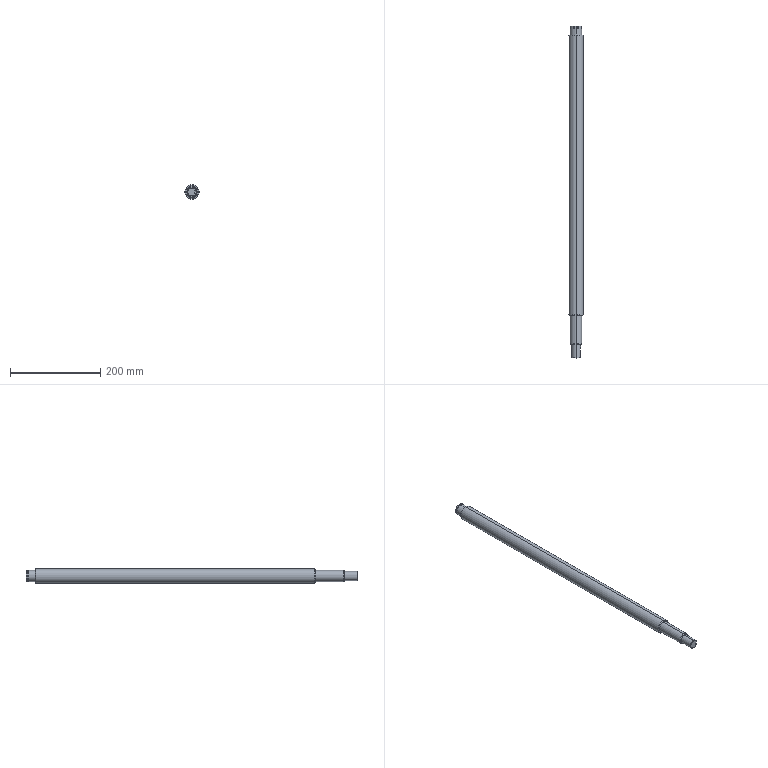Part | SolidWorks | features ICE 4, Chamfer 1, RevCut 1, Revolution 1 | 1 solid | 34 faces | box 32 x 734 x 32 mm | volume 548270 mm3 | cylinder 13 | cone 11 | plane 10 | commonest cylinder face diameters 25 x6 20 x2 23.9 x2 32 x2 6 x1
STEP:
#1=CARTESIAN_POINT('',(0.,344.5,11.5));
#2=VERTEX_POINT('',#1);
#3=CARTESIAN_POINT('',(0.,344.5,-11.5));
#4=VERTEX_POINT('',#3);
#5=CARTESIAN_POINT('',(0.,344.5,0.));
#6=DIRECTION('',(0.,1.,0.));
#7=DIRECTION('',(0.,0.,1.));
#8=AXIS2_PLACEMENT_3D('',#5,#6,#7);
#9=CIRCLE('',#8,11.5);
#10=EDGE_CURVE('',#2,#4,#9,.T.);
#11=ORIENTED_EDGE('',*,*,#10,.F.);
#12=CARTESIAN_POINT('',(0.,343.5,12.5));
#13=VERTEX_POINT('',#12);
#14=CARTESIAN_POINT('',(0.,344.5,11.5));
#15=DIRECTION('',(0.,-0.7071,0.7071));
#16=VECTOR('',#15,1000.);
#17=LINE('',#14,#16);
#18=EDGE_CURVE('',#2,#13,#17,.T.);
#19=ORIENTED_EDGE('',*,*,#18,.T.);
#20=CARTESIAN_POINT('',(0.,343.5,-12.5));
#21=VERTEX_POINT('',#20);
#22=CARTESIAN_POINT('',(0.,343.5,0.));
#23=DIRECTION('',(0.,-1.,0.));
#24=DIRECTION('',(0.,0.,1.));
#25=AXIS2_PLACEMENT_3D('',#22,#23,#24);
#26=CIRCLE('',#25,12.5);
#27=EDGE_CURVE('',#21,#13,#26,.T.);
#28=ORIENTED_EDGE('',*,*,#27,.F.);
#29=CARTESIAN_POINT('',(0.,344.5,-11.5));
#30=DIRECTION('',(0.,-0.7071,-0.7071));
#31=VECTOR('',#30,1000.);
#32=LINE('',#29,#31);
#33=EDGE_CURVE('',#4,#21,#32,.T.);
#34=ORIENTED_EDGE('',*,*,#33,.F.);
#35=EDGE_LOOP('',(#11,#19,#28,#34));
#36=FACE_OUTER_BOUND('',#35,.T.);
#37=CARTESIAN_POINT('',(0.,344.5,0.));
#38=DIRECTION('',(0.,-1.,0.));
#39=DIRECTION('',(0.,0.,-1.));
#40=AXIS2_PLACEMENT_3D('',#37,#38,#39);
#41=CONICAL_SURFACE('',#40,11.5,0.7854);
#42=ADVANCED_FACE('',(#36),#41,.T.);
#43=CARTESIAN_POINT('',(0.,324.5,15.));
#44=VERTEX_POINT('',#43);
#45=CARTESIAN_POINT('',(0.,324.5,-15.));
#46=VERTEX_POINT('',#45);
#47=CARTESIAN_POINT('',(0.,324.5,0.));
#48=DIRECTION('',(0.,1.,0.));
#49=DIRECTION('',(0.,0.,1.));
#50=AXIS2_PLACEMENT_3D('',#47,#48,#49);
#51=CIRCLE('',#50,15.);
#52=EDGE_CURVE('',#44,#46,#51,.T.);
#53=ORIENTED_EDGE('',*,*,#52,.F.);
#54=CARTESIAN_POINT('',(0.,323.5,16.));
#55=VERTEX_POINT('',#54);
#56=CARTESIAN_POINT('',(0.,324.5,15.));
#57=DIRECTION('',(0.,-0.7071,0.7071));
#58=VECTOR('',#57,1000.);
#59=LINE('',#56,#58);
#60=EDGE_CURVE('',#44,#55,#59,.T.);
#61=ORIENTED_EDGE('',*,*,#60,.T.);
#62=CARTESIAN_POINT('',(0.,323.5,-16.));
#63=VERTEX_POINT('',#62);
#64=CARTESIAN_POINT('',(0.,323.5,0.));
#65=DIRECTION('',(0.,-1.,0.));
#66=DIRECTION('',(0.,0.,1.));
#67=AXIS2_PLACEMENT_3D('',#64,#65,#66);
#68=CIRCLE('',#67,16.);
#69=EDGE_CURVE('',#63,#55,#68,.T.);
#70=ORIENTED_EDGE('',*,*,#69,.F.);
#71=CARTESIAN_POINT('',(0.,324.5,-15.));
#72=DIRECTION('',(0.,-0.7071,-0.7071));
#73=VECTOR('',#72,1000.);
#74=LINE('',#71,#73);
#75=EDGE_CURVE('',#46,#63,#74,.T.);
#76=ORIENTED_EDGE('',*,*,#75,.F.);
#77=EDGE_LOOP('',(#53,#61,#70,#76));
#78=FACE_OUTER_BOUND('',#77,.T.);
#79=CARTESIAN_POINT('',(0.,324.5,0.));
#80=DIRECTION('',(0.,-1.,0.));
#81=DIRECTION('',(0.,0.,-1.));
#82=AXIS2_PLACEMENT_3D('',#79,#80,#81);
#83=CONICAL_SURFACE('',#82,15.,0.7854);
#84=ADVANCED_FACE('',(#78),#83,.T.);
#85=CARTESIAN_POINT('',(0.,-294.5,-15.));
#86=VERTEX_POINT('',#85);
#87=CARTESIAN_POINT('',(0.,-294.5,15.));
#88=VERTEX_POINT('',#87);
#89=CARTESIAN_POINT('',(0.,-294.5,0.));
#90=DIRECTION('',(0.,-1.,0.));
#91=DIRECTION('',(0.,0.,-1.));
#92=AXIS2_PLACEMENT_3D('',#89,#90,#91);
#93=CIRCLE('',#92,15.);
#94=EDGE_CURVE('',#86,#88,#93,.T.);
#95=ORIENTED_EDGE('',*,*,#94,.F.);
#96=CARTESIAN_POINT('',(0.,-293.5,-16.));
#97=VERTEX_POINT('',#96);
#98=CARTESIAN_POINT('',(0.,-293.5,-16.));
#99=DIRECTION('',(0.,0.7071,-0.7071));
#100=VECTOR('',#99,1000.);
#101=LINE('',#98,#100);
#102=EDGE_CURVE('',#86,#97,#101,.T.);
#103=ORIENTED_EDGE('',*,*,#102,.T.);
#104=CARTESIAN_POINT('',(0.,-293.5,16.));
#105=VERTEX_POINT('',#104);
#106=CARTESIAN_POINT('',(0.,-293.5,0.));
#107=DIRECTION('',(0.,1.,0.));
#108=DIRECTION('',(0.,0.,-1.));
#109=AXIS2_PLACEMENT_3D('',#106,#107,#108);
#110=CIRCLE('',#109,16.);
#111=EDGE_CURVE('',#105,#97,#110,.T.);
#112=ORIENTED_EDGE('',*,*,#111,.F.);
#113=CARTESIAN_POINT('',(0.,-293.5,16.));
#114=DIRECTION('',(0.,0.7071,0.7071));
#115=VECTOR('',#114,1000.);
#116=LINE('',#113,#115);
#117=EDGE_CURVE('',#88,#105,#116,.T.);
#118=ORIENTED_EDGE('',*,*,#117,.F.);
#119=EDGE_LOOP('',(#95,#103,#112,#118));
#120=FACE_OUTER_BOUND('',#119,.T.);
#121=CARTESIAN_POINT('',(0.,-293.5,0.));
#122=DIRECTION('',(0.,1.,0.));
#123=DIRECTION('',(0.,0.,1.));
#124=AXIS2_PLACEMENT_3D('',#121,#122,#123);
#125=CONICAL_SURFACE('',#124,16.,0.7854);
#126=ADVANCED_FACE('',(#120),#125,.T.);
#127=CARTESIAN_POINT('',(0.,-359.5,-11.5));
#128=VERTEX_POINT('',#127);
#129=CARTESIAN_POINT('',(0.,-359.5,11.5));
#130=VERTEX_POINT('',#129);
#131=CARTESIAN_POINT('',(0.,-359.5,0.));
#132=DIRECTION('',(0.,-1.,0.));
#133=DIRECTION('',(0.,0.,-1.));
#134=AXIS2_PLACEMENT_3D('',#131,#132,#133);
#135=CIRCLE('',#134,11.5);
#136=EDGE_CURVE('',#128,#130,#135,.T.);
#137=ORIENTED_EDGE('',*,*,#136,.F.);
#138=CARTESIAN_POINT('',(0.,-358.5,-12.5));
#139=VERTEX_POINT('',#138);
#140=CARTESIAN_POINT('',(0.,-359.5,-11.5));
#141=DIRECTION('',(0.,0.7071,-0.7071));
#142=VECTOR('',#141,1000.);
#143=LINE('',#140,#142);
#144=EDGE_CURVE('',#128,#139,#143,.T.);
#145=ORIENTED_EDGE('',*,*,#144,.T.);
#146=CARTESIAN_POINT('',(0.,-358.5,12.5));
#147=VERTEX_POINT('',#146);
#148=CARTESIAN_POINT('',(0.,-358.5,0.));
#149=DIRECTION('',(0.,1.,0.));
#150=DIRECTION('',(0.,0.,-1.));
#151=AXIS2_PLACEMENT_3D('',#148,#149,#150);
#152=CIRCLE('',#151,12.5);
#153=EDGE_CURVE('',#147,#139,#152,.T.);
#154=ORIENTED_EDGE('',*,*,#153,.F.);
#155=CARTESIAN_POINT('',(0.,-359.5,11.5));
#156=DIRECTION('',(0.,0.7071,0.7071));
#157=VECTOR('',#156,1000.);
#158=LINE('',#155,#157);
#159=EDGE_CURVE('',#130,#147,#158,.T.);
#160=ORIENTED_EDGE('',*,*,#159,.F.);
#161=EDGE_LOOP('',(#137,#145,#154,#160));
#162=FACE_OUTER_BOUND('',#161,.T.);
#163=CARTESIAN_POINT('',(0.,-359.5,0.));
#164=DIRECTION('',(0.,1.,0.));
#165=DIRECTION('',(0.,0.,1.));
#166=AXIS2_PLACEMENT_3D('',#163,#164,#165);
#167=CONICAL_SURFACE('',#166,11.5,0.7854);
#168=ADVANCED_FACE('',(#162),#167,.T.);
#169=CARTESIAN_POINT('',(0.,-389.5,-9.));
#170=VERTEX_POINT('',#169);
#171=CARTESIAN_POINT('',(8.485,-389.5,-3.));
#172=VERTEX_POINT('',#171);
#173=CARTESIAN_POINT('',(0.,-389.5,0.));
#174=DIRECTION('',(0.,-1.,0.));
#175=DIRECTION('',(0.,0.,-1.));
#176=AXIS2_PLACEMENT_3D('',#173,#174,#175);
#177=CIRCLE('',#176,9.);
#178=EDGE_CURVE('',#170,#172,#177,.T.);
#179=ORIENTED_EDGE('',*,*,#178,.F.);
#180=CARTESIAN_POINT('',(0.,-388.5,-10.));
#181=VERTEX_POINT('',#180);
#182=CARTESIAN_POINT('',(0.,-389.5,-9.));
#183=DIRECTION('',(0.,0.7071,-0.7071));
#184=VECTOR('',#183,1000.);
#185=LINE('',#182,#184);
#186=EDGE_CURVE('',#170,#181,#185,.T.);
#187=ORIENTED_EDGE('',*,*,#186,.T.);
#188=CARTESIAN_POINT('',(9.539,-388.5,-3.));
#189=VERTEX_POINT('',#188);
#190=CARTESIAN_POINT('',(0.,-388.5,0.));
#191=DIRECTION('',(0.,1.,0.));
#192=DIRECTION('',(0.,0.,-1.));
#193=AXIS2_PLACEMENT_3D('',#190,#191,#192);
#194=CIRCLE('',#193,10.);
#195=EDGE_CURVE('',#189,#181,#194,.T.);
#196=ORIENTED_EDGE('',*,*,#195,.F.);
#197=CARTESIAN_POINT('',(8.485,-389.5,-3.));
#198=CARTESIAN_POINT('',(8.838,-389.168,-3.));
#199=CARTESIAN_POINT('',(9.189,-388.834,-3.));
#200=CARTESIAN_POINT('',(9.539,-388.5,-3.));
#201=B_SPLINE_CURVE_WITH_KNOTS('',3,(#197,#198,#199,#200),.UNSPECIFIED.,.F.,.F.,(4,4),(0.006491,0.007944),.UNSPECIFIED.);
#202=EDGE_CURVE('',#172,#189,#201,.T.);
#203=ORIENTED_EDGE('',*,*,#202,.F.);
#204=EDGE_LOOP('',(#179,#187,#196,#203));
#205=FACE_OUTER_BOUND('',#204,.T.);
#206=CARTESIAN_POINT('',(0.,-389.5,0.));
#207=DIRECTION('',(0.,1.,0.));
#208=DIRECTION('',(0.,0.,1.));
#209=AXIS2_PLACEMENT_3D('',#206,#207,#208);
#210=CONICAL_SURFACE('',#209,9.,0.7854);
#211=ADVANCED_FACE('',(#205),#210,.T.);
#212=ORIENTED_EDGE('',*,*,#186,.F.);
#213=CARTESIAN_POINT('',(0.,-389.5,9.));
#214=VERTEX_POINT('',#213);
#215=CARTESIAN_POINT('',(0.,-389.5,0.));
#216=DIRECTION('',(0.,-1.,0.));
#217=DIRECTION('',(0.,0.,-1.));
#218=AXIS2_PLACEMENT_3D('',#215,#216,#217);
#219=CIRCLE('',#218,9.);
#220=EDGE_CURVE('',#214,#170,#219,.T.);
#221=ORIENTED_EDGE('',*,*,#220,.F.);
#222=CARTESIAN_POINT('',(0.,-388.5,10.));
#223=VERTEX_POINT('',#222);
#224=CARTESIAN_POINT('',(0.,-389.5,9.));
#225=DIRECTION('',(0.,0.7071,0.7071));
#226=VECTOR('',#225,1000.);
#227=LINE('',#224,#226);
#228=EDGE_CURVE('',#214,#223,#227,.T.);
#229=ORIENTED_EDGE('',*,*,#228,.T.);
#230=CARTESIAN_POINT('',(0.,-388.5,0.));
#231=DIRECTION('',(0.,1.,0.));
#232=DIRECTION('',(0.,0.,-1.));
#233=AXIS2_PLACEMENT_3D('',#230,#231,#232);
#234=CIRCLE('',#233,10.);
#235=EDGE_CURVE('',#181,#223,#234,.T.);
#236=ORIENTED_EDGE('',*,*,#235,.F.);
#237=EDGE_LOOP('',(#212,#221,#229,#236));
#238=FACE_OUTER_BOUND('',#237,.T.);
#239=CARTESIAN_POINT('',(0.,-389.5,0.));
#240=DIRECTION('',(0.,1.,0.));
#241=DIRECTION('',(0.,0.,1.));
#242=AXIS2_PLACEMENT_3D('',#239,#240,#241);
#243=CONICAL_SURFACE('',#242,9.,0.7854);
#244=ADVANCED_FACE('',(#238),#243,.T.);
#245=ORIENTED_EDGE('',*,*,#27,.T.);
#246=CARTESIAN_POINT('',(0.,340.85,12.5));
#247=VERTEX_POINT('',#246);
#248=CARTESIAN_POINT('',(0.,344.5,12.5));
#249=DIRECTION('',(0.,-1.,0.));
#250=VECTOR('',#249,1000.);
#251=LINE('',#248,#250);
#252=EDGE_CURVE('',#13,#247,#251,.T.);
#253=ORIENTED_EDGE('',*,*,#252,.T.);
#254=CARTESIAN_POINT('',(0.,340.85,-12.5));
#255=VERTEX_POINT('',#254);
#256=CARTESIAN_POINT('',(0.,340.85,0.));
#257=DIRECTION('',(0.,1.,0.));
#258=DIRECTION('',(0.,0.,1.));
#259=AXIS2_PLACEMENT_3D('',#256,#257,#258);
#260=CIRCLE('',#259,12.5);
#261=EDGE_CURVE('',#247,#255,#260,.T.);
#262=ORIENTED_EDGE('',*,*,#261,.T.);
#263=CARTESIAN_POINT('',(0.,344.5,-12.5));
#264=DIRECTION('',(0.,-1.,0.));
#265=VECTOR('',#264,1000.);
#266=LINE('',#263,#265);
#267=EDGE_CURVE('',#21,#255,#266,.T.);
#268=ORIENTED_EDGE('',*,*,#267,.F.);
#269=EDGE_LOOP('',(#245,#253,#262,#268));
#270=FACE_OUTER_BOUND('',#269,.T.);
#271=CARTESIAN_POINT('',(0.,344.5,0.));
#272=DIRECTION('',(0.,-1.,0.));
#273=DIRECTION('',(0.,0.,-1.));
#274=AXIS2_PLACEMENT_3D('',#271,#272,#273);
#275=CYLINDRICAL_SURFACE('',#274,12.5);
#276=ADVANCED_FACE('',(#270),#275,.T.);
#277=CARTESIAN_POINT('',(0.,340.85,-11.95));
#278=VERTEX_POINT('',#277);
#279=CARTESIAN_POINT('',(0.,340.85,11.95));
#280=VERTEX_POINT('',#279);
#281=CARTESIAN_POINT('',(0.,340.85,0.));
#282=DIRECTION('',(0.,-1.,0.));
#283=DIRECTION('',(0.,0.,-1.));
#284=AXIS2_PLACEMENT_3D('',#281,#282,#283);
#285=CIRCLE('',#284,11.95);
#286=EDGE_CURVE('',#278,#280,#285,.T.);
#287=ORIENTED_EDGE('',*,*,#286,.T.);
#288=CARTESIAN_POINT('',(0.,339.5,11.95));
#289=VERTEX_POINT('',#288);
#290=CARTESIAN_POINT('',(0.,0.,11.95));
#291=DIRECTION('',(0.,-1.,0.));
#292=VECTOR('',#291,1000.);
#293=LINE('',#290,#292);
#294=EDGE_CURVE('',#280,#289,#293,.T.);
#295=ORIENTED_EDGE('',*,*,#294,.T.);
#296=CARTESIAN_POINT('',(0.,339.5,-11.95));
#297=VERTEX_POINT('',#296);
#298=CARTESIAN_POINT('',(0.,339.5,0.));
#299=DIRECTION('',(0.,-1.,0.));
#300=DIRECTION('',(0.,0.,-1.));
#301=AXIS2_PLACEMENT_3D('',#298,#299,#300);
#302=CIRCLE('',#301,11.95);
#303=EDGE_CURVE('',#297,#289,#302,.T.);
#304=ORIENTED_EDGE('',*,*,#303,.F.);
#305=CARTESIAN_POINT('',(0.,0.,-11.95));
#306=DIRECTION('',(0.,-1.,0.));
#307=VECTOR('',#306,1000.);
#308=LINE('',#305,#307);
#309=EDGE_CURVE('',#278,#297,#308,.T.);
#310=ORIENTED_EDGE('',*,*,#309,.F.);
#311=EDGE_LOOP('',(#287,#295,#304,#310));
#312=FACE_OUTER_BOUND('',#311,.T.);
#313=CARTESIAN_POINT('',(0.,0.,0.));
#314=DIRECTION('',(0.,-1.,0.));
#315=DIRECTION('',(0.,0.,-1.));
#316=AXIS2_PLACEMENT_3D('',#313,#314,#315);
#317=CYLINDRICAL_SURFACE('',#316,11.95);
#318=ADVANCED_FACE('',(#312),#317,.T.);
#319=ORIENTED_EDGE('',*,*,#195,.T.);
#320=CARTESIAN_POINT('',(0.,-359.5,-10.));
#321=VERTEX_POINT('',#320);
#322=CARTESIAN_POINT('',(0.,-389.5,-10.));
#323=DIRECTION('',(0.,1.,0.));
#324=VECTOR('',#323,1000.);
#325=LINE('',#322,#324);
#326=EDGE_CURVE('',#181,#321,#325,.T.);
#327=ORIENTED_EDGE('',*,*,#326,.T.);
#328=CARTESIAN_POINT('',(0.,-359.5,10.));
#329=VERTEX_POINT('',#328);
#330=CARTESIAN_POINT('',(0.,-359.5,0.));
#331=DIRECTION('',(0.,-1.,0.));
#332=DIRECTION('',(0.,0.,-1.));
#333=AXIS2_PLACEMENT_3D('',#330,#331,#332);
#334=CIRCLE('',#333,10.);
#335=EDGE_CURVE('',#321,#329,#334,.T.);
#336=ORIENTED_EDGE('',*,*,#335,.T.);
#337=CARTESIAN_POINT('',(0.,-389.5,10.));
#338=DIRECTION('',(0.,1.,0.));
#339=VECTOR('',#338,1000.);
#340=LINE('',#337,#339);
#341=EDGE_CURVE('',#223,#329,#340,.T.);
#342=ORIENTED_EDGE('',*,*,#341,.F.);
#343=CARTESIAN_POINT('',(9.539,-388.5,3.));
#344=VERTEX_POINT('',#343);
#345=CARTESIAN_POINT('',(0.,-388.5,0.));
#346=DIRECTION('',(0.,1.,0.));
#347=DIRECTION('',(0.,0.,-1.));
#348=AXIS2_PLACEMENT_3D('',#345,#346,#347);
#349=CIRCLE('',#348,10.);
#350=EDGE_CURVE('',#223,#344,#349,.T.);
#351=ORIENTED_EDGE('',*,*,#350,.T.);
#352=CARTESIAN_POINT('',(9.539,-369.5,3.));
#353=VERTEX_POINT('',#352);
#354=CARTESIAN_POINT('',(9.539,-389.5,3.));
#355=DIRECTION('',(0.,1.,0.));
#356=VECTOR('',#355,1000.);
#357=LINE('',#354,#356);
#358=EDGE_CURVE('',#344,#353,#357,.T.);
#359=ORIENTED_EDGE('',*,*,#358,.T.);
#360=CARTESIAN_POINT('',(9.539,-369.5,-3.));
#361=VERTEX_POINT('',#360);
#362=CARTESIAN_POINT('',(9.539,-369.5,3.));
#363=CARTESIAN_POINT('',(9.539,-369.301,3.));
#364=CARTESIAN_POINT('',(9.546,-369.105,2.98));
#365=CARTESIAN_POINT('',(9.569,-368.72,2.903));
#366=CARTESIAN_POINT('',(9.587,-368.529,2.845));
#367=CARTESIAN_POINT('',(9.631,-368.166,2.694));
#368=CARTESIAN_POINT('',(9.656,-367.994,2.602));
#369=CARTESIAN_POINT('',(9.712,-367.669,2.385));
#370=CARTESIAN_POINT('',(9.743,-367.516,2.259));
#371=CARTESIAN_POINT('',(9.832,-367.104,1.847));
#372=CARTESIAN_POINT('',(9.891,-366.881,1.514));
#373=CARTESIAN_POINT('',(9.954,-366.656,0.9732));
#374=CARTESIAN_POINT('',(9.971,-366.597,0.783));
#375=CARTESIAN_POINT('',(9.994,-366.52,0.3953));
#376=CARTESIAN_POINT('',(10.,-366.5,0.1999));
#377=CARTESIAN_POINT('',(10.,-366.5,-0.194));
#378=CARTESIAN_POINT('',(9.994,-366.519,-0.394));
#379=CARTESIAN_POINT('',(9.971,-366.596,-0.7797));
#380=CARTESIAN_POINT('',(9.955,-366.653,-0.9673));
#381=CARTESIAN_POINT('',(9.913,-366.805,-1.332));
#382=CARTESIAN_POINT('',(9.887,-366.898,-1.506));
#383=CARTESIAN_POINT('',(9.833,-367.114,-1.83));
#384=CARTESIAN_POINT('',(9.803,-367.24,-1.982));
#385=CARTESIAN_POINT('',(9.743,-367.516,-2.259));
#386=CARTESIAN_POINT('',(9.713,-367.667,-2.383));
#387=CARTESIAN_POINT('',(9.657,-367.99,-2.6));
#388=CARTESIAN_POINT('',(9.631,-368.166,-2.694));
#389=CARTESIAN_POINT('',(9.587,-368.527,-2.845));
#390=CARTESIAN_POINT('',(9.57,-368.714,-2.902));
#391=CARTESIAN_POINT('',(9.546,-369.101,-2.98));
#392=CARTESIAN_POINT('',(9.539,-369.301,-3.));
#393=CARTESIAN_POINT('',(9.539,-369.5,-3.));
#394=B_SPLINE_CURVE_WITH_KNOTS('',3,(#362,#363,#364,#365,#366,#367,#368,#369,#370,#371,#372,#373,#374,#375,#376,#377,#378,#379,#380,#381,#382,#383,#384,#385,#386,#387,#388,#389,#390,#391,#392,#393),.UNSPECIFIED.,.F.,.F.,(4,2,2,2,2,2,2,2,2,2,2,2,2,2,2,4),(0.,0.0005894,0.001179,0.001768,0.002358,0.003536,0.004126,0.004715,0.005305,0.005894,0.006484,0.007073,0.007662,0.008252,0.008841,0.009431),.UNSPECIFIED.);
#395=EDGE_CURVE('',#353,#361,#394,.T.);
#396=ORIENTED_EDGE('',*,*,#395,.T.);
#397=CARTESIAN_POINT('',(9.539,-389.5,-3.));
#398=DIRECTION('',(0.,-1.,0.));
#399=VECTOR('',#398,1000.);
#400=LINE('',#397,#399);
#401=EDGE_CURVE('',#361,#189,#400,.T.);
#402=ORIENTED_EDGE('',*,*,#401,.T.);
#403=EDGE_LOOP('',(#319,#327,#336,#342,#351,#359,#396,#402));
#404=FACE_OUTER_BOUND('',#403,.T.);
#405=CARTESIAN_POINT('',(0.,-389.5,0.));
#406=DIRECTION('',(0.,1.,0.));
#407=DIRECTION('',(0.,0.,1.));
#408=AXIS2_PLACEMENT_3D('',#405,#406,#407);
#409=CYLINDRICAL_SURFACE('',#408,10.);
#410=ADVANCED_FACE('',(#404),#409,.T.);
#411=ORIENTED_EDGE('',*,*,#153,.T.);
#412=CARTESIAN_POINT('',(0.,-294.5,-12.5));
#413=VERTEX_POINT('',#412);
#414=CARTESIAN_POINT('',(0.,-359.5,-12.5));
#415=DIRECTION('',(0.,1.,0.));
#416=VECTOR('',#415,1000.);
#417=LINE('',#414,#416);
#418=EDGE_CURVE('',#139,#413,#417,.T.);
#419=ORIENTED_EDGE('',*,*,#418,.T.);
#420=CARTESIAN_POINT('',(0.,-294.5,12.5));
#421=VERTEX_POINT('',#420);
#422=CARTESIAN_POINT('',(0.,-294.5,0.));
#423=DIRECTION('',(0.,-1.,0.));
#424=DIRECTION('',(0.,0.,-1.));
#425=AXIS2_PLACEMENT_3D('',#422,#423,#424);
#426=CIRCLE('',#425,12.5);
#427=EDGE_CURVE('',#413,#421,#426,.T.);
#428=ORIENTED_EDGE('',*,*,#427,.T.);
#429=CARTESIAN_POINT('',(0.,-359.5,12.5));
#430=DIRECTION('',(0.,1.,0.));
#431=VECTOR('',#430,1000.);
#432=LINE('',#429,#431);
#433=EDGE_CURVE('',#147,#421,#432,.T.);
#434=ORIENTED_EDGE('',*,*,#433,.F.);
#435=EDGE_LOOP('',(#411,#419,#428,#434));
#436=FACE_OUTER_BOUND('',#435,.T.);
#437=CARTESIAN_POINT('',(0.,-359.5,0.));
#438=DIRECTION('',(0.,1.,0.));
#439=DIRECTION('',(0.,0.,1.));
#440=AXIS2_PLACEMENT_3D('',#437,#438,#439);
#441=CYLINDRICAL_SURFACE('',#440,12.5);
#442=ADVANCED_FACE('',(#436),#441,.T.);
#443=ORIENTED_EDGE('',*,*,#111,.T.);
#444=CARTESIAN_POINT('',(0.,-294.5,-16.));
#445=DIRECTION('',(0.,1.,0.));
#446=VECTOR('',#445,1000.);
#447=LINE('',#444,#446);
#448=EDGE_CURVE('',#97,#63,#447,.T.);
#449=ORIENTED_EDGE('',*,*,#448,.T.);
#450=ORIENTED_EDGE('',*,*,#69,.T.);
#451=CARTESIAN_POINT('',(0.,-294.5,16.));
#452=DIRECTION('',(0.,1.,0.));
#453=VECTOR('',#452,1000.);
#454=LINE('',#451,#453);
#455=EDGE_CURVE('',#105,#55,#454,.T.);
#456=ORIENTED_EDGE('',*,*,#455,.F.);
#457=EDGE_LOOP('',(#443,#449,#450,#456));
#458=FACE_OUTER_BOUND('',#457,.T.);
#459=CARTESIAN_POINT('',(0.,-294.5,0.));
#460=DIRECTION('',(0.,1.,0.));
#461=DIRECTION('',(0.,0.,1.));
#462=AXIS2_PLACEMENT_3D('',#459,#460,#461);
#463=CYLINDRICAL_SURFACE('',#462,16.);
#464=ADVANCED_FACE('',(#458),#463,.T.);
#465=CARTESIAN_POINT('',(0.,339.5,-12.5));
#466=VERTEX_POINT('',#465);
#467=CARTESIAN_POINT('',(0.,339.5,12.5));
#468=VERTEX_POINT('',#467);
#469=CARTESIAN_POINT('',(0.,339.5,0.));
#470=DIRECTION('',(0.,-1.,0.));
#471=DIRECTION('',(0.,0.,-1.));
#472=AXIS2_PLACEMENT_3D('',#469,#470,#471);
#473=CIRCLE('',#472,12.5);
#474=EDGE_CURVE('',#466,#468,#473,.T.);
#475=ORIENTED_EDGE('',*,*,#474,.T.);
#476=CARTESIAN_POINT('',(0.,324.5,12.5));
#477=VERTEX_POINT('',#476);
#478=CARTESIAN_POINT('',(0.,344.5,12.5));
#479=DIRECTION('',(0.,-1.,0.));
#480=VECTOR('',#479,1000.);
#481=LINE('',#478,#480);
#482=EDGE_CURVE('',#468,#477,#481,.T.);
#483=ORIENTED_EDGE('',*,*,#482,.T.);
#484=CARTESIAN_POINT('',(0.,324.5,-12.5));
#485=VERTEX_POINT('',#484);
#486=CARTESIAN_POINT('',(0.,324.5,0.));
#487=DIRECTION('',(0.,1.,0.));
#488=DIRECTION('',(0.,0.,1.));
#489=AXIS2_PLACEMENT_3D('',#486,#487,#488);
#490=CIRCLE('',#489,12.5);
#491=EDGE_CURVE('',#477,#485,#490,.T.);
#492=ORIENTED_EDGE('',*,*,#491,.T.);
#493=CARTESIAN_POINT('',(0.,344.5,-12.5));
#494=DIRECTION('',(0.,-1.,0.));
#495=VECTOR('',#494,1000.);
#496=LINE('',#493,#495);
#497=EDGE_CURVE('',#466,#485,#496,.T.);
#498=ORIENTED_EDGE('',*,*,#497,.F.);
#499=EDGE_LOOP('',(#475,#483,#492,#498));
#500=FACE_OUTER_BOUND('',#499,.T.);
#501=CARTESIAN_POINT('',(0.,344.5,0.));
#502=DIRECTION('',(0.,-1.,0.));
#503=DIRECTION('',(0.,0.,-1.));
#504=AXIS2_PLACEMENT_3D('',#501,#502,#503);
#505=CYLINDRICAL_SURFACE('',#504,12.5);
#506=ADVANCED_FACE('',(#500),#505,.T.);
#507=ORIENTED_EDGE('',*,*,#482,.F.);
#508=CARTESIAN_POINT('',(0.,339.5,0.));
#509=DIRECTION('',(0.,-1.,0.));
#510=DIRECTION('',(0.,0.,-1.));
#511=AXIS2_PLACEMENT_3D('',#508,#509,#510);
#512=CIRCLE('',#511,12.5);
#513=EDGE_CURVE('',#468,#466,#512,.T.);
#514=ORIENTED_EDGE('',*,*,#513,.T.);
#515=ORIENTED_EDGE('',*,*,#497,.T.);
#516=CARTESIAN_POINT('',(0.,324.5,0.));
#517=DIRECTION('',(0.,1.,0.));
#518=DIRECTION('',(0.,0.,1.));
#519=AXIS2_PLACEMENT_3D('',#516,#517,#518);
#520=CIRCLE('',#519,12.5);
#521=EDGE_CURVE('',#485,#477,#520,.T.);
#522=ORIENTED_EDGE('',*,*,#521,.T.);
#523=EDGE_LOOP('',(#507,#514,#515,#522));
#524=FACE_OUTER_BOUND('',#523,.T.);
#525=CARTESIAN_POINT('',(0.,344.5,0.));
#526=DIRECTION('',(0.,-1.,0.));
#527=DIRECTION('',(0.,0.,-1.));
#528=AXIS2_PLACEMENT_3D('',#525,#526,#527);
#529=CYLINDRICAL_SURFACE('',#528,12.5);
#530=ADVANCED_FACE('',(#524),#529,.T.);
#531=CARTESIAN_POINT('',(0.,324.5,0.));
#532=DIRECTION('',(0.,1.,0.));
#533=DIRECTION('',(0.,0.,1.));
#534=AXIS2_PLACEMENT_3D('',#531,#532,#533);
#535=CIRCLE('',#534,15.);
#536=EDGE_CURVE('',#46,#44,#535,.T.);
#537=ORIENTED_EDGE('',*,*,#536,.T.);
#538=ORIENTED_EDGE('',*,*,#52,.T.);
#539=EDGE_LOOP('',(#537,#538));
#540=FACE_OUTER_BOUND('',#539,.T.);
#541=ORIENTED_EDGE('',*,*,#521,.F.);
#542=ORIENTED_EDGE('',*,*,#491,.F.);
#543=EDGE_LOOP('',(#541,#542));
#544=FACE_BOUND('',#543,.T.);
#545=CARTESIAN_POINT('',(0.,324.5,0.));
#546=DIRECTION('',(0.,1.,0.));
#547=DIRECTION('',(0.,0.,1.));
#548=AXIS2_PLACEMENT_3D('',#545,#546,#547);
#549=PLANE('',#548);
#550=ADVANCED_FACE('',(#540,#544),#549,.T.);
#551=CARTESIAN_POINT('',(0.,-359.5,0.));
#552=DIRECTION('',(0.,-1.,0.));
#553=DIRECTION('',(0.,0.,-1.));
#554=AXIS2_PLACEMENT_3D('',#551,#552,#553);
#555=CIRCLE('',#554,11.5);
#556=EDGE_CURVE('',#130,#128,#555,.T.);
#557=ORIENTED_EDGE('',*,*,#556,.T.);
#558=ORIENTED_EDGE('',*,*,#136,.T.);
#559=EDGE_LOOP('',(#557,#558));
#560=FACE_OUTER_BOUND('',#559,.T.);
#561=CARTESIAN_POINT('',(0.,-359.5,0.));
#562=DIRECTION('',(0.,-1.,0.));
#563=DIRECTION('',(0.,0.,-1.));
#564=AXIS2_PLACEMENT_3D('',#561,#562,#563);
#565=CIRCLE('',#564,10.);
#566=EDGE_CURVE('',#329,#321,#565,.T.);
#567=ORIENTED_EDGE('',*,*,#566,.F.);
#568=ORIENTED_EDGE('',*,*,#335,.F.);
#569=EDGE_LOOP('',(#567,#568));
#570=FACE_BOUND('',#569,.T.);
#571=CARTESIAN_POINT('',(0.,-359.5,0.));
#572=DIRECTION('',(0.,-1.,0.));
#573=DIRECTION('',(0.,0.,-1.));
#574=AXIS2_PLACEMENT_3D('',#571,#572,#573);
#575=PLANE('',#574);
#576=ADVANCED_FACE('',(#560,#570),#575,.T.);
#577=CARTESIAN_POINT('',(0.,-294.5,0.));
#578=DIRECTION('',(0.,-1.,0.));
#579=DIRECTION('',(0.,0.,-1.));
#580=AXIS2_PLACEMENT_3D('',#577,#578,#579);
#581=CIRCLE('',#580,15.);
#582=EDGE_CURVE('',#88,#86,#581,.T.);
#583=ORIENTED_EDGE('',*,*,#582,.T.);
#584=ORIENTED_EDGE('',*,*,#94,.T.);
#585=EDGE_LOOP('',(#583,#584));
#586=FACE_OUTER_BOUND('',#585,.T.);
#587=CARTESIAN_POINT('',(0.,-294.5,0.));
#588=DIRECTION('',(0.,-1.,0.));
#589=DIRECTION('',(0.,0.,-1.));
#590=AXIS2_PLACEMENT_3D('',#587,#588,#589);
#591=CIRCLE('',#590,12.5);
#592=EDGE_CURVE('',#421,#413,#591,.T.);
#593=ORIENTED_EDGE('',*,*,#592,.F.);
#594=ORIENTED_EDGE('',*,*,#427,.F.);
#595=EDGE_LOOP('',(#593,#594));
#596=FACE_BOUND('',#595,.T.);
#597=CARTESIAN_POINT('',(16.,-294.5,0.));
#598=DIRECTION('',(0.,-1.,0.));
#599=DIRECTION('',(0.,0.,-1.));
#600=AXIS2_PLACEMENT_3D('',#597,#598,#599);
#601=PLANE('',#600);
#602=ADVANCED_FACE('',(#586,#596),#601,.T.);
#603=ORIENTED_EDGE('',*,*,#448,.F.);
#604=CARTESIAN_POINT('',(0.,-293.5,0.));
#605=DIRECTION('',(0.,1.,0.));
#606=DIRECTION('',(0.,0.,-1.));
#607=AXIS2_PLACEMENT_3D('',#604,#605,#606);
#608=CIRCLE('',#607,16.);
#609=EDGE_CURVE('',#97,#105,#608,.T.);
#610=ORIENTED_EDGE('',*,*,#609,.T.);
#611=ORIENTED_EDGE('',*,*,#455,.T.);
#612=CARTESIAN_POINT('',(0.,323.5,0.));
#613=DIRECTION('',(0.,-1.,0.));
#614=DIRECTION('',(0.,0.,1.));
#615=AXIS2_PLACEMENT_3D('',#612,#613,#614);
#616=CIRCLE('',#615,16.);
#617=EDGE_CURVE('',#55,#63,#616,.T.);
#618=ORIENTED_EDGE('',*,*,#617,.T.);
#619=EDGE_LOOP('',(#603,#610,#611,#618));
#620=FACE_OUTER_BOUND('',#619,.T.);
#621=CARTESIAN_POINT('',(0.,-294.5,0.));
#622=DIRECTION('',(0.,1.,0.));
#623=DIRECTION('',(0.,0.,1.));
#624=AXIS2_PLACEMENT_3D('',#621,#622,#623);
#625=CYLINDRICAL_SURFACE('',#624,16.);
#626=ADVANCED_FACE('',(#620),#625,.T.);
#627=ORIENTED_EDGE('',*,*,#418,.F.);
#628=CARTESIAN_POINT('',(0.,-358.5,0.));
#629=DIRECTION('',(0.,1.,0.));
#630=DIRECTION('',(0.,0.,-1.));
#631=AXIS2_PLACEMENT_3D('',#628,#629,#630);
#632=CIRCLE('',#631,12.5);
#633=EDGE_CURVE('',#139,#147,#632,.T.);
#634=ORIENTED_EDGE('',*,*,#633,.T.);
#635=ORIENTED_EDGE('',*,*,#433,.T.);
#636=ORIENTED_EDGE('',*,*,#592,.T.);
#637=EDGE_LOOP('',(#627,#634,#635,#636));
#638=FACE_OUTER_BOUND('',#637,.T.);
#639=CARTESIAN_POINT('',(0.,-359.5,0.));
#640=DIRECTION('',(0.,1.,0.));
#641=DIRECTION('',(0.,0.,1.));
#642=AXIS2_PLACEMENT_3D('',#639,#640,#641);
#643=CYLINDRICAL_SURFACE('',#642,12.5);
#644=ADVANCED_FACE('',(#638),#643,.T.);
#645=ORIENTED_EDGE('',*,*,#326,.F.);
#646=ORIENTED_EDGE('',*,*,#235,.T.);
#647=ORIENTED_EDGE('',*,*,#341,.T.);
#648=ORIENTED_EDGE('',*,*,#566,.T.);
#649=EDGE_LOOP('',(#645,#646,#647,#648));
#650=FACE_OUTER_BOUND('',#649,.T.);
#651=CARTESIAN_POINT('',(0.,-389.5,0.));
#652=DIRECTION('',(0.,1.,0.));
#653=DIRECTION('',(0.,0.,1.));
#654=AXIS2_PLACEMENT_3D('',#651,#652,#653);
#655=CYLINDRICAL_SURFACE('',#654,10.);
#656=ADVANCED_FACE('',(#650),#655,.T.);
#657=CARTESIAN_POINT('',(6.5,-389.5,-3.));
#658=VERTEX_POINT('',#657);
#659=CARTESIAN_POINT('',(0.,-389.5,-3.));
#660=DIRECTION('',(1.,0.,0.));
#661=VECTOR('',#660,1000.);
#662=LINE('',#659,#661);
#663=EDGE_CURVE('',#658,#172,#662,.T.);
#664=ORIENTED_EDGE('',*,*,#663,.F.);
#665=CARTESIAN_POINT('',(6.5,-389.5,3.));
#666=VERTEX_POINT('',#665);
#667=CARTESIAN_POINT('',(6.5,-389.5,0.));
#668=DIRECTION('',(0.,0.,1.));
#669=VECTOR('',#668,1000.);
#670=LINE('',#667,#669);
#671=EDGE_CURVE('',#658,#666,#670,.T.);
#672=ORIENTED_EDGE('',*,*,#671,.T.);
#673=CARTESIAN_POINT('',(8.485,-389.5,3.));
#674=VERTEX_POINT('',#673);
#675=CARTESIAN_POINT('',(0.,-389.5,3.));
#676=DIRECTION('',(-1.,0.,0.));
#677=VECTOR('',#676,1000.);
#678=LINE('',#675,#677);
#679=EDGE_CURVE('',#674,#666,#678,.T.);
#680=ORIENTED_EDGE('',*,*,#679,.F.);
#681=CARTESIAN_POINT('',(0.,-389.5,0.));
#682=DIRECTION('',(0.,-1.,0.));
#683=DIRECTION('',(0.,0.,-1.));
#684=AXIS2_PLACEMENT_3D('',#681,#682,#683);
#685=CIRCLE('',#684,9.);
#686=EDGE_CURVE('',#674,#214,#685,.T.);
#687=ORIENTED_EDGE('',*,*,#686,.T.);
#688=ORIENTED_EDGE('',*,*,#220,.T.);
#689=ORIENTED_EDGE('',*,*,#178,.T.);
#690=EDGE_LOOP('',(#664,#672,#680,#687,#688,#689));
#691=FACE_OUTER_BOUND('',#690,.T.);
#692=CARTESIAN_POINT('',(0.,-389.5,0.));
#693=DIRECTION('',(0.,-1.,0.));
#694=DIRECTION('',(0.,0.,-1.));
#695=AXIS2_PLACEMENT_3D('',#692,#693,#694);
#696=PLANE('',#695);
#697=ADVANCED_FACE('',(#691),#696,.T.);
#698=ORIENTED_EDGE('',*,*,#303,.T.);
#699=CARTESIAN_POINT('',(0.,339.5,0.));
#700=DIRECTION('',(0.,-1.,0.));
#701=DIRECTION('',(0.,0.,-1.));
#702=AXIS2_PLACEMENT_3D('',#699,#700,#701);
#703=CIRCLE('',#702,11.95);
#704=EDGE_CURVE('',#289,#297,#703,.T.);
#705=ORIENTED_EDGE('',*,*,#704,.T.);
#706=EDGE_LOOP('',(#698,#705));
#707=FACE_BOUND('',#706,.T.);
#708=ORIENTED_EDGE('',*,*,#474,.F.);
#709=ORIENTED_EDGE('',*,*,#513,.F.);
#710=EDGE_LOOP('',(#708,#709));
#711=FACE_OUTER_BOUND('',#710,.T.);
#712=CARTESIAN_POINT('',(-25.853,339.5,0.));
#713=DIRECTION('',(0.,-1.,0.));
#714=DIRECTION('',(0.,0.,-1.));
#715=AXIS2_PLACEMENT_3D('',#712,#713,#714);
#716=PLANE('',#715);
#717=ADVANCED_FACE('',(#707,#711),#716,.F.);
#718=ORIENTED_EDGE('',*,*,#286,.F.);
#719=CARTESIAN_POINT('',(0.,340.85,0.));
#720=DIRECTION('',(0.,-1.,0.));
#721=DIRECTION('',(0.,0.,-1.));
#722=AXIS2_PLACEMENT_3D('',#719,#720,#721);
#723=CIRCLE('',#722,11.95);
#724=EDGE_CURVE('',#280,#278,#723,.T.);
#725=ORIENTED_EDGE('',*,*,#724,.F.);
#726=EDGE_LOOP('',(#718,#725));
#727=FACE_BOUND('',#726,.T.);
#728=CARTESIAN_POINT('',(0.,340.85,0.));
#729=DIRECTION('',(0.,1.,0.));
#730=DIRECTION('',(0.,0.,1.));
#731=AXIS2_PLACEMENT_3D('',#728,#729,#730);
#732=CIRCLE('',#731,12.5);
#733=EDGE_CURVE('',#255,#247,#732,.T.);
#734=ORIENTED_EDGE('',*,*,#733,.F.);
#735=ORIENTED_EDGE('',*,*,#261,.F.);
#736=EDGE_LOOP('',(#734,#735));
#737=FACE_OUTER_BOUND('',#736,.T.);
#738=CARTESIAN_POINT('',(-25.853,340.85,0.));
#739=DIRECTION('',(0.,1.,0.));
#740=DIRECTION('',(0.,0.,1.));
#741=AXIS2_PLACEMENT_3D('',#738,#739,#740);
#742=PLANE('',#741);
#743=ADVANCED_FACE('',(#727,#737),#742,.F.);
#744=ORIENTED_EDGE('',*,*,#294,.F.);
#745=ORIENTED_EDGE('',*,*,#724,.T.);
#746=ORIENTED_EDGE('',*,*,#309,.T.);
#747=ORIENTED_EDGE('',*,*,#704,.F.);
#748=EDGE_LOOP('',(#744,#745,#746,#747));
#749=FACE_OUTER_BOUND('',#748,.T.);
#750=CARTESIAN_POINT('',(0.,0.,0.));
#751=DIRECTION('',(0.,-1.,0.));
#752=DIRECTION('',(0.,0.,-1.));
#753=AXIS2_PLACEMENT_3D('',#750,#751,#752);
#754=CYLINDRICAL_SURFACE('',#753,11.95);
#755=ADVANCED_FACE('',(#749),#754,.T.);
#756=CARTESIAN_POINT('',(0.,344.5,0.));
#757=DIRECTION('',(0.,1.,0.));
#758=DIRECTION('',(0.,0.,1.));
#759=AXIS2_PLACEMENT_3D('',#756,#757,#758);
#760=CIRCLE('',#759,11.5);
#761=EDGE_CURVE('',#4,#2,#760,.T.);
#762=ORIENTED_EDGE('',*,*,#761,.T.);
#763=ORIENTED_EDGE('',*,*,#10,.T.);
#764=EDGE_LOOP('',(#762,#763));
#765=FACE_OUTER_BOUND('',#764,.T.);
#766=CARTESIAN_POINT('',(0.,344.5,0.));
#767=DIRECTION('',(0.,1.,0.));
#768=DIRECTION('',(0.,0.,1.));
#769=AXIS2_PLACEMENT_3D('',#766,#767,#768);
#770=PLANE('',#769);
#771=ADVANCED_FACE('',(#765),#770,.T.);
#772=ORIENTED_EDGE('',*,*,#252,.F.);
#773=CARTESIAN_POINT('',(0.,343.5,0.));
#774=DIRECTION('',(0.,-1.,0.));
#775=DIRECTION('',(0.,0.,1.));
#776=AXIS2_PLACEMENT_3D('',#773,#774,#775);
#777=CIRCLE('',#776,12.5);
#778=EDGE_CURVE('',#13,#21,#777,.T.);
#779=ORIENTED_EDGE('',*,*,#778,.T.);
#780=ORIENTED_EDGE('',*,*,#267,.T.);
#781=ORIENTED_EDGE('',*,*,#733,.T.);
#782=EDGE_LOOP('',(#772,#779,#780,#781));
#783=FACE_OUTER_BOUND('',#782,.T.);
#784=CARTESIAN_POINT('',(0.,344.5,0.));
#785=DIRECTION('',(0.,-1.,0.));
#786=DIRECTION('',(0.,0.,-1.));
#787=AXIS2_PLACEMENT_3D('',#784,#785,#786);
#788=CYLINDRICAL_SURFACE('',#787,12.5);
#789=ADVANCED_FACE('',(#783),#788,.T.);
#790=ORIENTED_EDGE('',*,*,#228,.F.);
#791=ORIENTED_EDGE('',*,*,#686,.F.);
#792=CARTESIAN_POINT('',(9.539,-388.5,3.));
#793=CARTESIAN_POINT('',(9.189,-388.834,3.));
#794=CARTESIAN_POINT('',(8.838,-389.168,3.));
#795=CARTESIAN_POINT('',(8.485,-389.5,3.));
#796=B_SPLINE_CURVE_WITH_KNOTS('',3,(#792,#793,#794,#795),.UNSPECIFIED.,.F.,.F.,(4,4),(0.006016,0.007469),.UNSPECIFIED.);
#797=EDGE_CURVE('',#344,#674,#796,.T.);
#798=ORIENTED_EDGE('',*,*,#797,.F.);
#799=ORIENTED_EDGE('',*,*,#350,.F.);
#800=EDGE_LOOP('',(#790,#791,#798,#799));
#801=FACE_OUTER_BOUND('',#800,.T.);
#802=CARTESIAN_POINT('',(0.,-389.5,0.));
#803=DIRECTION('',(0.,1.,0.));
#804=DIRECTION('',(0.,0.,1.));
#805=AXIS2_PLACEMENT_3D('',#802,#803,#804);
#806=CONICAL_SURFACE('',#805,9.,0.7854);
#807=ADVANCED_FACE('',(#801),#806,.T.);
#808=ORIENTED_EDGE('',*,*,#144,.F.);
#809=ORIENTED_EDGE('',*,*,#556,.F.);
#810=ORIENTED_EDGE('',*,*,#159,.T.);
#811=ORIENTED_EDGE('',*,*,#633,.F.);
#812=EDGE_LOOP('',(#808,#809,#810,#811));
#813=FACE_OUTER_BOUND('',#812,.T.);
#814=CARTESIAN_POINT('',(0.,-359.5,0.));
#815=DIRECTION('',(0.,1.,0.));
#816=DIRECTION('',(0.,0.,1.));
#817=AXIS2_PLACEMENT_3D('',#814,#815,#816);
#818=CONICAL_SURFACE('',#817,11.5,0.7854);
#819=ADVANCED_FACE('',(#813),#818,.T.);
#820=ORIENTED_EDGE('',*,*,#102,.F.);
#821=ORIENTED_EDGE('',*,*,#582,.F.);
#822=ORIENTED_EDGE('',*,*,#117,.T.);
#823=ORIENTED_EDGE('',*,*,#609,.F.);
#824=EDGE_LOOP('',(#820,#821,#822,#823));
#825=FACE_OUTER_BOUND('',#824,.T.);
#826=CARTESIAN_POINT('',(0.,-293.5,0.));
#827=DIRECTION('',(0.,1.,0.));
#828=DIRECTION('',(0.,0.,1.));
#829=AXIS2_PLACEMENT_3D('',#826,#827,#828);
#830=CONICAL_SURFACE('',#829,16.,0.7854);
#831=ADVANCED_FACE('',(#825),#830,.T.);
#832=ORIENTED_EDGE('',*,*,#60,.F.);
#833=ORIENTED_EDGE('',*,*,#536,.F.);
#834=ORIENTED_EDGE('',*,*,#75,.T.);
#835=ORIENTED_EDGE('',*,*,#617,.F.);
#836=EDGE_LOOP('',(#832,#833,#834,#835));
#837=FACE_OUTER_BOUND('',#836,.T.);
#838=CARTESIAN_POINT('',(0.,324.5,0.));
#839=DIRECTION('',(0.,-1.,0.));
#840=DIRECTION('',(0.,0.,-1.));
#841=AXIS2_PLACEMENT_3D('',#838,#839,#840);
#842=CONICAL_SURFACE('',#841,15.,0.7854);
#843=ADVANCED_FACE('',(#837),#842,.T.);
#844=ORIENTED_EDGE('',*,*,#18,.F.);
#845=ORIENTED_EDGE('',*,*,#761,.F.);
#846=ORIENTED_EDGE('',*,*,#33,.T.);
#847=ORIENTED_EDGE('',*,*,#778,.F.);
#848=EDGE_LOOP('',(#844,#845,#846,#847));
#849=FACE_OUTER_BOUND('',#848,.T.);
#850=CARTESIAN_POINT('',(0.,344.5,0.));
#851=DIRECTION('',(0.,-1.,0.));
#852=DIRECTION('',(0.,0.,-1.));
#853=AXIS2_PLACEMENT_3D('',#850,#851,#852);
#854=CONICAL_SURFACE('',#853,11.5,0.7854);
#855=ADVANCED_FACE('',(#849),#854,.T.);
#856=CARTESIAN_POINT('',(6.5,-369.5,3.));
#857=VERTEX_POINT('',#856);
#858=CARTESIAN_POINT('',(6.5,-369.5,3.));
#859=DIRECTION('',(1.,0.,0.));
#860=VECTOR('',#859,1000.);
#861=LINE('',#858,#860);
#862=EDGE_CURVE('',#857,#353,#861,.T.);
#863=ORIENTED_EDGE('',*,*,#862,.F.);
#864=CARTESIAN_POINT('',(6.5,-369.5,-3.));
#865=VERTEX_POINT('',#864);
#866=CARTESIAN_POINT('',(6.5,-369.5,0.));
#867=DIRECTION('',(1.,0.,0.));
#868=DIRECTION('',(0.,0.,-1.));
#869=AXIS2_PLACEMENT_3D('',#866,#867,#868);
#870=CIRCLE('',#869,3.);
#871=EDGE_CURVE('',#865,#857,#870,.T.);
#872=ORIENTED_EDGE('',*,*,#871,.F.);
#873=CARTESIAN_POINT('',(6.5,-369.5,-3.));
#874=DIRECTION('',(1.,0.,0.));
#875=VECTOR('',#874,1000.);
#876=LINE('',#873,#875);
#877=EDGE_CURVE('',#865,#361,#876,.T.);
#878=ORIENTED_EDGE('',*,*,#877,.T.);
#879=ORIENTED_EDGE('',*,*,#395,.F.);
#880=EDGE_LOOP('',(#863,#872,#878,#879));
#881=FACE_OUTER_BOUND('',#880,.T.);
#882=CARTESIAN_POINT('',(6.5,-369.5,0.));
#883=DIRECTION('',(1.,0.,0.));
#884=DIRECTION('',(0.,0.,-1.));
#885=AXIS2_PLACEMENT_3D('',#882,#883,#884);
#886=CYLINDRICAL_SURFACE('',#885,3.);
#887=ADVANCED_FACE('',(#881),#886,.F.);
#888=ORIENTED_EDGE('',*,*,#877,.F.);
#889=CARTESIAN_POINT('',(6.5,-369.5,-3.));
#890=DIRECTION('',(0.,1.,0.));
#891=VECTOR('',#890,1000.);
#892=LINE('',#889,#891);
#893=EDGE_CURVE('',#658,#865,#892,.T.);
#894=ORIENTED_EDGE('',*,*,#893,.F.);
#895=ORIENTED_EDGE('',*,*,#663,.T.);
#896=ORIENTED_EDGE('',*,*,#202,.T.);
#897=ORIENTED_EDGE('',*,*,#401,.F.);
#898=EDGE_LOOP('',(#888,#894,#895,#896,#897));
#899=FACE_OUTER_BOUND('',#898,.T.);
#900=CARTESIAN_POINT('',(6.5,-369.5,-3.));
#901=DIRECTION('',(0.,0.,-1.));
#902=DIRECTION('',(0.,1.,0.));
#903=AXIS2_PLACEMENT_3D('',#900,#901,#902);
#904=PLANE('',#903);
#905=ADVANCED_FACE('',(#899),#904,.F.);
#906=ORIENTED_EDGE('',*,*,#797,.T.);
#907=ORIENTED_EDGE('',*,*,#679,.T.);
#908=CARTESIAN_POINT('',(6.5,-369.5,3.));
#909=DIRECTION('',(0.,-1.,0.));
#910=VECTOR('',#909,1000.);
#911=LINE('',#908,#910);
#912=EDGE_CURVE('',#857,#666,#911,.T.);
#913=ORIENTED_EDGE('',*,*,#912,.F.);
#914=ORIENTED_EDGE('',*,*,#862,.T.);
#915=ORIENTED_EDGE('',*,*,#358,.F.);
#916=EDGE_LOOP('',(#906,#907,#913,#914,#915));
#917=FACE_OUTER_BOUND('',#916,.T.);
#918=CARTESIAN_POINT('',(6.5,-369.5,3.));
#919=DIRECTION('',(0.,0.,1.));
#920=DIRECTION('',(0.,-1.,0.));
#921=AXIS2_PLACEMENT_3D('',#918,#919,#920);
#922=PLANE('',#921);
#923=ADVANCED_FACE('',(#917),#922,.F.);
#924=ORIENTED_EDGE('',*,*,#893,.T.);
#925=ORIENTED_EDGE('',*,*,#871,.T.);
#926=ORIENTED_EDGE('',*,*,#912,.T.);
#927=ORIENTED_EDGE('',*,*,#671,.F.);
#928=EDGE_LOOP('',(#924,#925,#926,#927));
#929=FACE_OUTER_BOUND('',#928,.T.);
#930=CARTESIAN_POINT('',(6.5,-369.5,0.));
#931=DIRECTION('',(1.,0.,0.));
#932=DIRECTION('',(0.,0.,-1.));
#933=AXIS2_PLACEMENT_3D('',#930,#931,#932);
#934=PLANE('',#933);
#935=ADVANCED_FACE('',(#929),#934,.T.);
#936=CLOSED_SHELL('',(#42,#84,#126,#168,#211,#244,#276,#318,#410,#442,#464,#506,#530,#550,#576,#602,#626,#644,#656,#697,#717,#743,#755,#771,#789,#807,#819,#831,#843,#855,#887,#905,#923,#935));
#937=MANIFOLD_SOLID_BREP('',#936);
#938=CARTESIAN_POINT('',(0.,0.,0.));
#939=DIRECTION('',(0.,0.,1.));
#940=DIRECTION('',(1.,0.,0.));
#941=AXIS2_PLACEMENT_3D('',#938,#939,#940);
#942=(LENGTH_UNIT()NAMED_UNIT(*)SI_UNIT(.MILLI.,.METRE.));
#943=UNCERTAINTY_MEASURE_WITH_UNIT(LENGTH_MEASURE(0.00001),#942,'','');
#944=(NAMED_UNIT(*)PLANE_ANGLE_UNIT()SI_UNIT($,.RADIAN.));
#945=(NAMED_UNIT(*)SI_UNIT($,.STERADIAN.)SOLID_ANGLE_UNIT());
#946=(GEOMETRIC_REPRESENTATION_CONTEXT(3)GLOBAL_UNCERTAINTY_ASSIGNED_CONTEXT((#943))GLOBAL_UNIT_ASSIGNED_CONTEXT((#942,#944,#945))REPRESENTATION_CONTEXT('',''));
#947=ADVANCED_BREP_SHAPE_REPRESENTATION('',(#937,#941),#946);